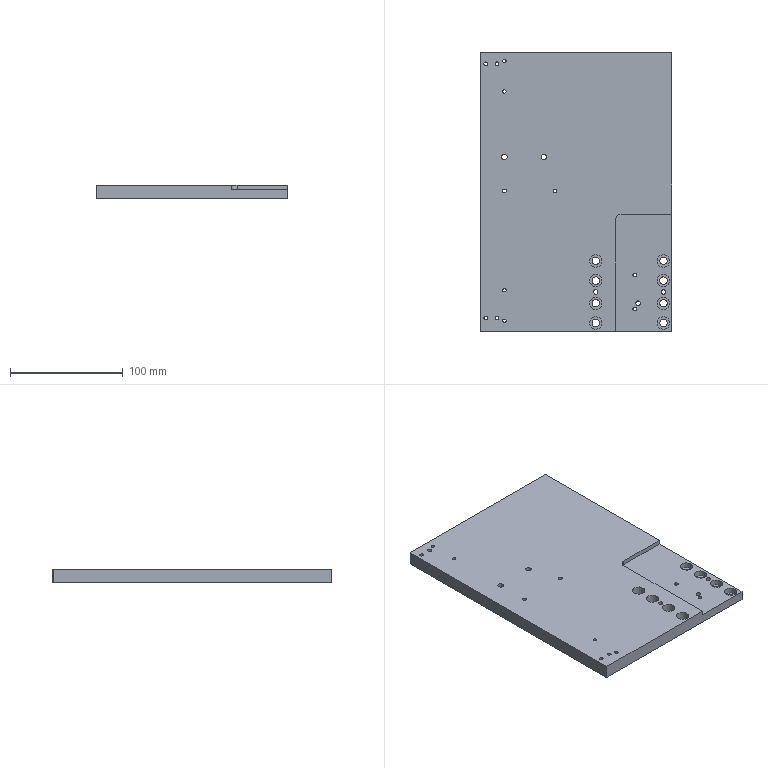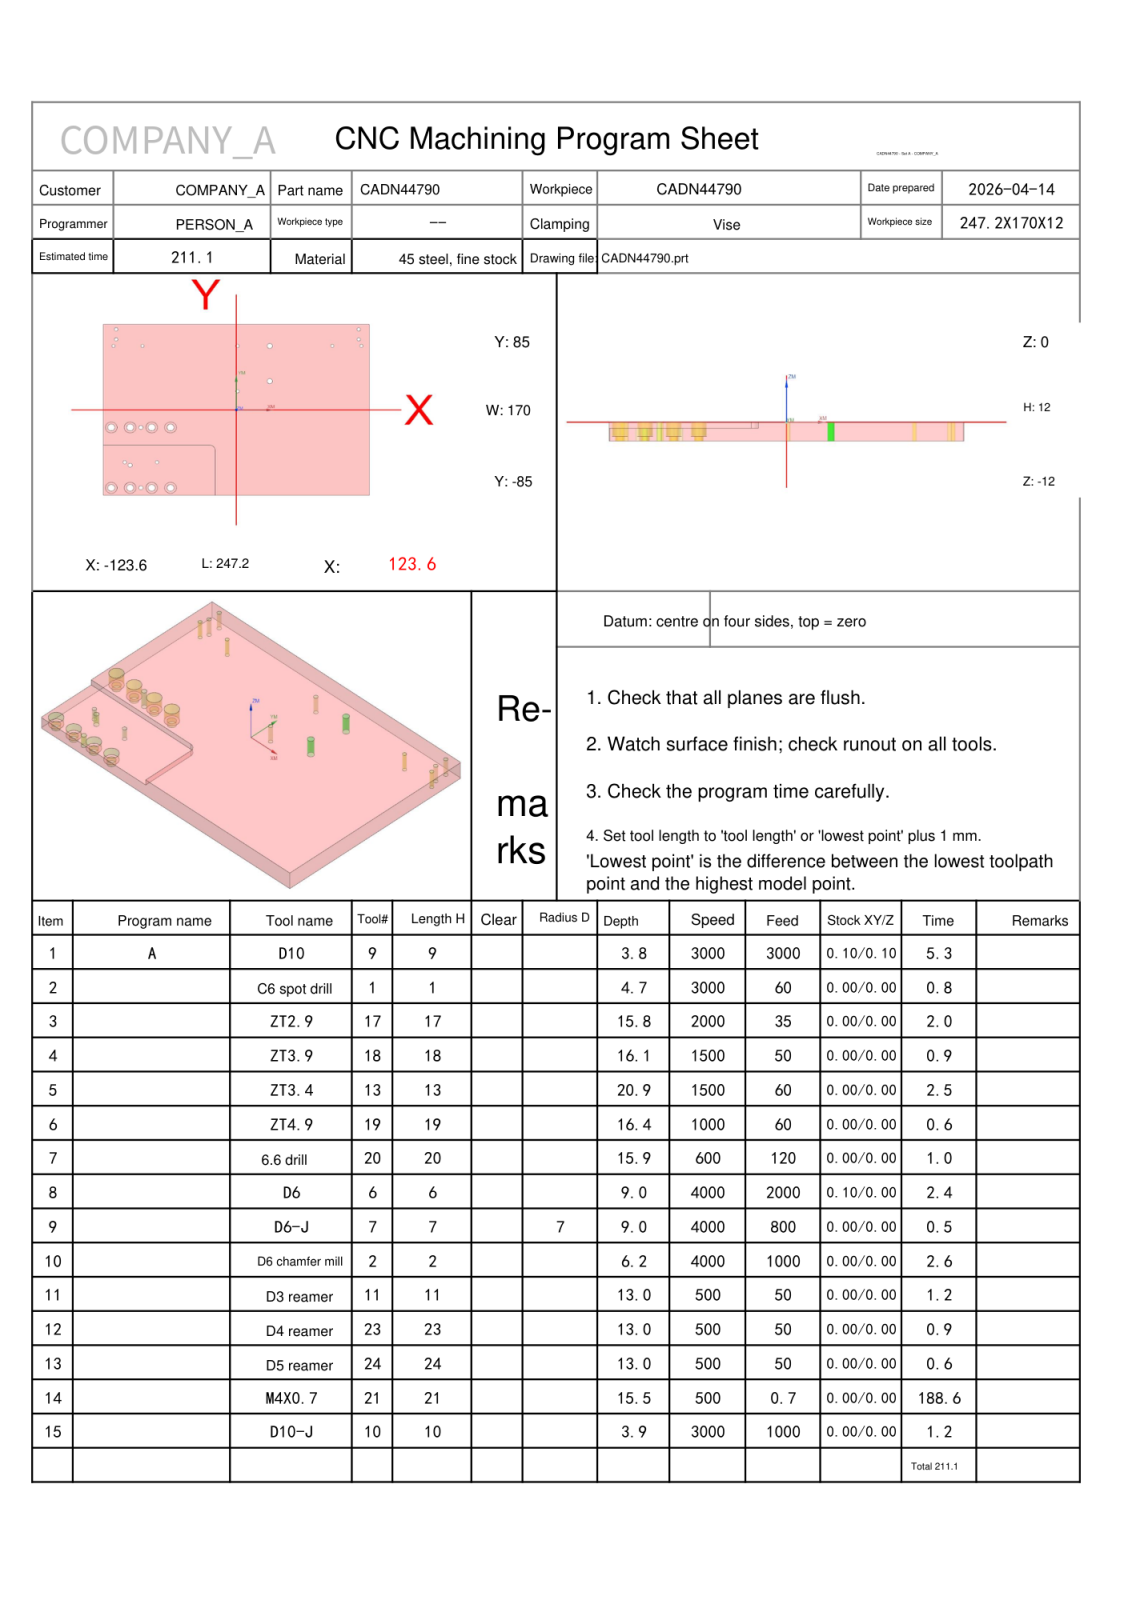NC program | NX | posted by the shop | part box 170 x 247.2 x 12 mm
Whole program, first 1507 of 2214 lines:
%
O0001
(Machine time: 390.98 MIN)
(===Total Tool:15===)
(T9=D10     D=10.  R=0.   D-  H09 Z=-3.8  )
(T1=C6 spot drill   D=6.   R=0.   D-  H01 Z=-4.7  )
(T17=ZT2.9  D=2.9  DR_a=120 D-  H17 Z=-15.84)
(T18=ZT3.9  D=3.9  DR_a=120 D-  H18 Z=-16.13)
(T13=ZT3.4  D=3.4  DR_a=118 D-  H13 Z=-20.9 )
(T19=ZT4.9  D=4.9  DR_a=120 D-  H19 Z=-16.41)
(T20=6.6 drill  D=6.6  DR_a=120 D-  H20 Z=-15.91)
(T6=D6      D=6.   R=0.   D-  H06 Z=-9.   )
(T7=D6-J    D=6.   R=0.   D7  H07 Z=-9.   )
(T2=D6 chamfer mill   D=6.   R=0.   D-  H02 Z=-6.2  )
(T11=D3 reamer   D=3.   DR_a=180 D-  H11 Z=-13.  )
(T23=D4 reamer   D=4.   DR_a=180 D-  H23 Z=-13.  )
(T24=D5 reamer   D=5.   DR_a=180 D-  H24 Z=-13.  )
(T21=M4X0.7 D=3.3  DR_a=180 D-  H21 Z=-15.5 )
(T10=D10-J  D=10.  R=0.   D10 H10 Z=-3.9  )
G80 G90 G17 G49 G40
G91 G28 Z0
M01
N1 T09 M06
(D10  D=10. R=0. H=09 ce=0.10 di=0.10)
G00 G90 G54 X-69.7 Y-93. M03 S3000
G43 H09 Z10.1
M08
Z1.3
G01 Z-.2 F3000.
Y-89.9
Y-86.195
G03 X-70.695 Y-85.2 I-1. J-.005
G01 X-127.501
G02 X-128.5 Y-84.201 I.001 J1.
G01 Y-78.699
G02 X-127.501 Y-77.7 I1. J-.001
G01 X-63.196
G02 X-62.2 Y-78.696 I-.004 J-1.
G01 Y-88.9
G03 X-61.2 Y-89.9 I1. J0.0
G01 X-55.7
G03 X-54.7 Y-88.9 I0.0 J1.
G01 Y-78.696
Y-71.196
G03 X-55.696 Y-70.2 I-1. J-.004
G01 X-127.501
G02 X-128.5 Y-69.201 I.001 J1.
G01 Y-63.699
G02 X-127.501 Y-62.7 I1. J-.001
G01 X-48.197
G02 X-47.2 Y-63.697 I-.003 J-1.
G01 Y-88.9
G03 X-46.2 Y-89.9 I1. J0.0
G01 X-40.7
G03 X-39.7 Y-88.9 I0.0 J1.
G01 Y-63.697
Y-56.197
G03 X-40.697 Y-55.2 I-1. J-.003
G01 X-127.501
G02 X-128.5 Y-54.201 I.001 J1.
G01 Y-48.699
G02 X-127.501 Y-47.7 I1. J-.001
G01 X-33.198
G02 X-32.2 Y-48.698 I-.002 J-1.
G01 Y-89.044
G03 X-31.354 Y-90.032 I1. J.001
G01 X-25.854 Y-90.888
X-25.7 Y-90.9
G03 X-24.7 Y-89.9 I0.0 J1.
G01 Y-40.2
X-128.5
X-131.7
Z1.3
G00 X-69.7 Y-93.
Z1.1
G01 Z-.4
Y-89.9
Y-86.195
G03 X-70.695 Y-85.2 I-1. J-.005
G01 X-127.501
G02 X-128.5 Y-84.201 I.001 J1.
G01 Y-78.699
G02 X-127.501 Y-77.7 I1. J-.001
G01 X-63.196
G02 X-62.2 Y-78.696 I-.004 J-1.
G01 Y-88.9
G03 X-61.2 Y-89.9 I1. J0.0
G01 X-55.7
G03 X-54.7 Y-88.9 I0.0 J1.
G01 Y-78.696
Y-71.196
G03 X-55.696 Y-70.2 I-1. J-.004
G01 X-127.501
G02 X-128.5 Y-69.201 I.001 J1.
G01 Y-63.699
G02 X-127.501 Y-62.7 I1. J-.001
G01 X-48.197
G02 X-47.2 Y-63.697 I-.003 J-1.
G01 Y-88.9
G03 X-46.2 Y-89.9 I1. J0.0
G01 X-40.7
G03 X-39.7 Y-88.9 I0.0 J1.
G01 Y-63.697
Y-56.197
G03 X-40.697 Y-55.2 I-1. J-.003
G01 X-127.501
G02 X-128.5 Y-54.201 I.001 J1.
G01 Y-48.699
G02 X-127.501 Y-47.7 I1. J-.001
G01 X-33.198
G02 X-32.2 Y-48.698 I-.002 J-1.
G01 Y-89.044
G03 X-31.354 Y-90.032 I1. J.001
G01 X-25.854 Y-90.888
X-25.7 Y-90.9
G03 X-24.7 Y-89.9 I0.0 J1.
G01 Y-40.2
X-128.5
X-131.7
Z1.1
G00 X-69.7 Y-93.
Z.9
G01 Z-.6
Y-89.9
Y-86.195
G03 X-70.695 Y-85.2 I-1. J-.005
G01 X-127.501
G02 X-128.5 Y-84.201 I.001 J1.
G01 Y-78.699
G02 X-127.501 Y-77.7 I1. J-.001
G01 X-63.196
G02 X-62.2 Y-78.696 I-.004 J-1.
G01 Y-88.9
G03 X-61.2 Y-89.9 I1. J0.0
G01 X-55.7
G03 X-54.7 Y-88.9 I0.0 J1.
G01 Y-78.696
Y-71.196
G03 X-55.696 Y-70.2 I-1. J-.004
G01 X-127.501
G02 X-128.5 Y-69.201 I.001 J1.
G01 Y-63.699
G02 X-127.501 Y-62.7 I1. J-.001
G01 X-48.197
G02 X-47.2 Y-63.697 I-.003 J-1.
G01 Y-88.9
G03 X-46.2 Y-89.9 I1. J0.0
G01 X-40.7
G03 X-39.7 Y-88.9 I0.0 J1.
G01 Y-63.697
Y-56.197
G03 X-40.697 Y-55.2 I-1. J-.003
G01 X-127.501
G02 X-128.5 Y-54.201 I.001 J1.
G01 Y-48.699
G02 X-127.501 Y-47.7 I1. J-.001
G01 X-33.198
G02 X-32.2 Y-48.698 I-.002 J-1.
G01 Y-89.044
G03 X-31.354 Y-90.032 I1. J.001
G01 X-25.854 Y-90.888
X-25.7 Y-90.9
G03 X-24.7 Y-89.9 I0.0 J1.
G01 Y-40.2
X-128.5
X-131.7
Z.9
G00 X-69.7 Y-93.
Z.7
G01 Z-.8
Y-89.9
Y-86.195
G03 X-70.695 Y-85.2 I-1. J-.005
G01 X-127.501
G02 X-128.5 Y-84.201 I.001 J1.
G01 Y-78.699
G02 X-127.501 Y-77.7 I1. J-.001
G01 X-63.196
G02 X-62.2 Y-78.696 I-.004 J-1.
G01 Y-88.9
G03 X-61.2 Y-89.9 I1. J0.0
G01 X-55.7
G03 X-54.7 Y-88.9 I0.0 J1.
G01 Y-78.696
Y-71.196
G03 X-55.696 Y-70.2 I-1. J-.004
G01 X-127.501
G02 X-128.5 Y-69.201 I.001 J1.
G01 Y-63.699
G02 X-127.501 Y-62.7 I1. J-.001
G01 X-48.197
G02 X-47.2 Y-63.697 I-.003 J-1.
G01 Y-88.9
G03 X-46.2 Y-89.9 I1. J0.0
G01 X-40.7
G03 X-39.7 Y-88.9 I0.0 J1.
G01 Y-63.697
Y-56.197
G03 X-40.697 Y-55.2 I-1. J-.003
G01 X-127.501
G02 X-128.5 Y-54.201 I.001 J1.
G01 Y-48.699
G02 X-127.501 Y-47.7 I1. J-.001
G01 X-33.198
G02 X-32.2 Y-48.698 I-.002 J-1.
G01 Y-89.044
G03 X-31.354 Y-90.032 I1. J.001
G01 X-25.854 Y-90.888
X-25.7 Y-90.9
G03 X-24.7 Y-89.9 I0.0 J1.
G01 Y-40.2
X-128.5
X-131.7
Z.7
G00 X-69.7 Y-93.
Z.5
G01 Z-1.
Y-89.9
Y-86.195
G03 X-70.695 Y-85.2 I-1. J-.005
G01 X-127.501
G02 X-128.5 Y-84.201 I.001 J1.
G01 Y-78.699
G02 X-127.501 Y-77.7 I1. J-.001
G01 X-63.196
G02 X-62.2 Y-78.696 I-.004 J-1.
G01 Y-88.9
G03 X-61.2 Y-89.9 I1. J0.0
G01 X-55.7
G03 X-54.7 Y-88.9 I0.0 J1.
G01 Y-78.696
Y-71.196
G03 X-55.696 Y-70.2 I-1. J-.004
G01 X-127.501
G02 X-128.5 Y-69.201 I.001 J1.
G01 Y-63.699
G02 X-127.501 Y-62.7 I1. J-.001
G01 X-48.197
G02 X-47.2 Y-63.697 I-.003 J-1.
G01 Y-88.9
G03 X-46.2 Y-89.9 I1. J0.0
G01 X-40.7
G03 X-39.7 Y-88.9 I0.0 J1.
G01 Y-63.697
Y-56.197
G03 X-40.697 Y-55.2 I-1. J-.003
G01 X-127.501
G02 X-128.5 Y-54.201 I.001 J1.
G01 Y-48.699
G02 X-127.501 Y-47.7 I1. J-.001
G01 X-33.198
G02 X-32.2 Y-48.698 I-.002 J-1.
G01 Y-89.044
G03 X-31.354 Y-90.032 I1. J.001
G01 X-25.854 Y-90.888
X-25.7 Y-90.9
G03 X-24.7 Y-89.9 I0.0 J1.
G01 Y-40.2
X-128.5
X-131.7
Z.5
G00 X-69.7 Y-93.
Z.3
G01 Z-1.2
Y-89.9
Y-86.195
G03 X-70.695 Y-85.2 I-1. J-.005
G01 X-127.501
G02 X-128.5 Y-84.201 I.001 J1.
G01 Y-78.699
G02 X-127.501 Y-77.7 I1. J-.001
G01 X-63.196
G02 X-62.2 Y-78.696 I-.004 J-1.
G01 Y-88.9
G03 X-61.2 Y-89.9 I1. J0.0
G01 X-55.7
G03 X-54.7 Y-88.9 I0.0 J1.
G01 Y-78.696
Y-71.196
G03 X-55.696 Y-70.2 I-1. J-.004
G01 X-127.501
G02 X-128.5 Y-69.201 I.001 J1.
G01 Y-63.699
G02 X-127.501 Y-62.7 I1. J-.001
G01 X-48.197
G02 X-47.2 Y-63.697 I-.003 J-1.
G01 Y-88.9
G03 X-46.2 Y-89.9 I1. J0.0
G01 X-40.7
G03 X-39.7 Y-88.9 I0.0 J1.
G01 Y-63.697
Y-56.197
G03 X-40.697 Y-55.2 I-1. J-.003
G01 X-127.501
G02 X-128.5 Y-54.201 I.001 J1.
G01 Y-48.699
G02 X-127.501 Y-47.7 I1. J-.001
G01 X-33.198
G02 X-32.2 Y-48.698 I-.002 J-1.
G01 Y-89.044
G03 X-31.354 Y-90.032 I1. J.001
G01 X-25.854 Y-90.888
X-25.7 Y-90.9
G03 X-24.7 Y-89.9 I0.0 J1.
G01 Y-40.2
X-128.5
X-131.7
Z.3
G00 X-69.7 Y-93.
Z.1
G01 Z-1.4
Y-89.9
Y-86.195
G03 X-70.695 Y-85.2 I-1. J-.005
G01 X-127.501
G02 X-128.5 Y-84.201 I.001 J1.
G01 Y-78.699
G02 X-127.501 Y-77.7 I1. J-.001
G01 X-63.196
G02 X-62.2 Y-78.696 I-.004 J-1.
G01 Y-88.9
G03 X-61.2 Y-89.9 I1. J0.0
G01 X-55.7
G03 X-54.7 Y-88.9 I0.0 J1.
G01 Y-78.696
Y-71.196
G03 X-55.696 Y-70.2 I-1. J-.004
G01 X-127.501
G02 X-128.5 Y-69.201 I.001 J1.
G01 Y-63.699
G02 X-127.501 Y-62.7 I1. J-.001
G01 X-48.197
G02 X-47.2 Y-63.697 I-.003 J-1.
G01 Y-88.9
G03 X-46.2 Y-89.9 I1. J0.0
G01 X-40.7
G03 X-39.7 Y-88.9 I0.0 J1.
G01 Y-63.697
Y-56.197
G03 X-40.697 Y-55.2 I-1. J-.003
G01 X-127.501
G02 X-128.5 Y-54.201 I.001 J1.
G01 Y-48.699
G02 X-127.501 Y-47.7 I1. J-.001
G01 X-33.198
G02 X-32.2 Y-48.698 I-.002 J-1.
G01 Y-89.044
G03 X-31.354 Y-90.032 I1. J.001
G01 X-25.854 Y-90.888
X-25.7 Y-90.9
G03 X-24.7 Y-89.9 I0.0 J1.
G01 Y-40.2
X-128.5
X-131.7
Z.1
G00 X-69.7 Y-93.
Z-.1
G01 Z-1.6
Y-89.9
Y-86.195
G03 X-70.695 Y-85.2 I-1. J-.005
G01 X-127.501
G02 X-128.5 Y-84.201 I.001 J1.
G01 Y-78.699
G02 X-127.501 Y-77.7 I1. J-.001
G01 X-63.196
G02 X-62.2 Y-78.696 I-.004 J-1.
G01 Y-88.9
G03 X-61.2 Y-89.9 I1. J0.0
G01 X-55.7
G03 X-54.7 Y-88.9 I0.0 J1.
G01 Y-78.696
Y-71.196
G03 X-55.696 Y-70.2 I-1. J-.004
G01 X-127.501
G02 X-128.5 Y-69.201 I.001 J1.
G01 Y-63.699
G02 X-127.501 Y-62.7 I1. J-.001
G01 X-48.197
G02 X-47.2 Y-63.697 I-.003 J-1.
G01 Y-88.9
G03 X-46.2 Y-89.9 I1. J0.0
G01 X-40.7
G03 X-39.7 Y-88.9 I0.0 J1.
G01 Y-63.697
Y-56.197
G03 X-40.697 Y-55.2 I-1. J-.003
G01 X-127.501
G02 X-128.5 Y-54.201 I.001 J1.
G01 Y-48.699
G02 X-127.501 Y-47.7 I1. J-.001
G01 X-33.198
G02 X-32.2 Y-48.698 I-.002 J-1.
G01 Y-89.044
G03 X-31.354 Y-90.032 I1. J.001
G01 X-25.854 Y-90.888
X-25.7 Y-90.9
G03 X-24.7 Y-89.9 I0.0 J1.
G01 Y-40.2
X-128.5
X-131.7
Z-.1
G00 X-69.7 Y-93.
Z-.3
G01 Z-1.8
Y-89.9
Y-86.195
G03 X-70.695 Y-85.2 I-1. J-.005
G01 X-127.501
G02 X-128.5 Y-84.201 I.001 J1.
G01 Y-78.699
G02 X-127.501 Y-77.7 I1. J-.001
G01 X-63.196
G02 X-62.2 Y-78.696 I-.004 J-1.
G01 Y-88.9
G03 X-61.2 Y-89.9 I1. J0.0
G01 X-55.7
G03 X-54.7 Y-88.9 I0.0 J1.
G01 Y-78.696
Y-71.196
G03 X-55.696 Y-70.2 I-1. J-.004
G01 X-127.501
G02 X-128.5 Y-69.201 I.001 J1.
G01 Y-63.699
G02 X-127.501 Y-62.7 I1. J-.001
G01 X-48.197
G02 X-47.2 Y-63.697 I-.003 J-1.
G01 Y-88.9
G03 X-46.2 Y-89.9 I1. J0.0
G01 X-40.7
G03 X-39.7 Y-88.9 I0.0 J1.
G01 Y-63.697
Y-56.197
G03 X-40.697 Y-55.2 I-1. J-.003
G01 X-127.501
G02 X-128.5 Y-54.201 I.001 J1.
G01 Y-48.699
G02 X-127.501 Y-47.7 I1. J-.001
G01 X-33.198
G02 X-32.2 Y-48.698 I-.002 J-1.
G01 Y-89.044
G03 X-31.354 Y-90.032 I1. J.001
G01 X-25.854 Y-90.888
X-25.7 Y-90.9
G03 X-24.7 Y-89.9 I0.0 J1.
G01 Y-40.2
X-128.5
X-131.7
Z-.3
G00 X-69.7 Y-93.
Z-.5
G01 Z-2.
Y-89.9
Y-86.195
G03 X-70.695 Y-85.2 I-1. J-.005
G01 X-127.501
G02 X-128.5 Y-84.201 I.001 J1.
G01 Y-78.699
G02 X-127.501 Y-77.7 I1. J-.001
G01 X-63.196
G02 X-62.2 Y-78.696 I-.004 J-1.
G01 Y-88.9
G03 X-61.2 Y-89.9 I1. J0.0
G01 X-55.7
G03 X-54.7 Y-88.9 I0.0 J1.
G01 Y-78.696
Y-71.196
G03 X-55.696 Y-70.2 I-1. J-.004
G01 X-127.501
G02 X-128.5 Y-69.201 I.001 J1.
G01 Y-63.699
G02 X-127.501 Y-62.7 I1. J-.001
G01 X-48.197
G02 X-47.2 Y-63.697 I-.003 J-1.
G01 Y-88.9
G03 X-46.2 Y-89.9 I1. J0.0
G01 X-40.7
G03 X-39.7 Y-88.9 I0.0 J1.
G01 Y-63.697
Y-56.197
G03 X-40.697 Y-55.2 I-1. J-.003
G01 X-127.501
G02 X-128.5 Y-54.201 I.001 J1.
G01 Y-48.699
G02 X-127.501 Y-47.7 I1. J-.001
G01 X-33.198
G02 X-32.2 Y-48.698 I-.002 J-1.
G01 Y-89.044
G03 X-31.354 Y-90.032 I1. J.001
G01 X-25.854 Y-90.888
X-25.7 Y-90.9
G03 X-24.7 Y-89.9 I0.0 J1.
G01 Y-40.2
X-128.5
X-131.7
Z-.5
G00 X-69.7 Y-93.
Z-.7
G01 Z-2.2
Y-89.9
Y-86.195
G03 X-70.695 Y-85.2 I-1. J-.005
G01 X-127.501
G02 X-128.5 Y-84.201 I.001 J1.
G01 Y-78.699
G02 X-127.501 Y-77.7 I1. J-.001
G01 X-63.196
G02 X-62.2 Y-78.696 I-.004 J-1.
G01 Y-88.9
G03 X-61.2 Y-89.9 I1. J0.0
G01 X-55.7
G03 X-54.7 Y-88.9 I0.0 J1.
G01 Y-78.696
Y-71.196
G03 X-55.696 Y-70.2 I-1. J-.004
G01 X-127.501
G02 X-128.5 Y-69.201 I.001 J1.
G01 Y-63.699
G02 X-127.501 Y-62.7 I1. J-.001
G01 X-48.197
G02 X-47.2 Y-63.697 I-.003 J-1.
G01 Y-88.9
G03 X-46.2 Y-89.9 I1. J0.0
G01 X-40.7
G03 X-39.7 Y-88.9 I0.0 J1.
G01 Y-63.697
Y-56.197
G03 X-40.697 Y-55.2 I-1. J-.003
G01 X-127.501
G02 X-128.5 Y-54.201 I.001 J1.
G01 Y-48.699
G02 X-127.501 Y-47.7 I1. J-.001
G01 X-33.198
G02 X-32.2 Y-48.698 I-.002 J-1.
G01 Y-89.044
G03 X-31.354 Y-90.032 I1. J.001
G01 X-25.854 Y-90.888
X-25.7 Y-90.9
G03 X-24.7 Y-89.9 I0.0 J1.
G01 Y-40.2
X-128.5
X-131.7
Z-.7
G00 X-69.7 Y-93.
Z-.9
G01 Z-2.4
Y-89.9
Y-86.195
G03 X-70.695 Y-85.2 I-1. J-.005
G01 X-127.501
G02 X-128.5 Y-84.201 I.001 J1.
G01 Y-78.699
G02 X-127.501 Y-77.7 I1. J-.001
G01 X-63.196
G02 X-62.2 Y-78.696 I-.004 J-1.
G01 Y-88.9
G03 X-61.2 Y-89.9 I1. J0.0
G01 X-55.7
G03 X-54.7 Y-88.9 I0.0 J1.
G01 Y-78.696
Y-71.196
G03 X-55.696 Y-70.2 I-1. J-.004
G01 X-127.501
G02 X-128.5 Y-69.201 I.001 J1.
G01 Y-63.699
G02 X-127.501 Y-62.7 I1. J-.001
G01 X-48.197
G02 X-47.2 Y-63.697 I-.003 J-1.
G01 Y-88.9
G03 X-46.2 Y-89.9 I1. J0.0
G01 X-40.7
G03 X-39.7 Y-88.9 I0.0 J1.
G01 Y-63.697
Y-56.197
G03 X-40.697 Y-55.2 I-1. J-.003
G01 X-127.501
G02 X-128.5 Y-54.201 I.001 J1.
G01 Y-48.699
G02 X-127.501 Y-47.7 I1. J-.001
G01 X-33.198
G02 X-32.2 Y-48.698 I-.002 J-1.
G01 Y-89.044
G03 X-31.354 Y-90.032 I1. J.001
G01 X-25.854 Y-90.888
X-25.7 Y-90.9
G03 X-24.7 Y-89.9 I0.0 J1.
G01 Y-40.2
X-128.5
X-131.7
Z-.9
G00 X-69.7 Y-93.
Z-1.1
G01 Z-2.6
Y-89.9
Y-86.195
G03 X-70.695 Y-85.2 I-1. J-.005
G01 X-127.501
G02 X-128.5 Y-84.201 I.001 J1.
G01 Y-78.699
G02 X-127.501 Y-77.7 I1. J-.001
G01 X-63.196
G02 X-62.2 Y-78.696 I-.004 J-1.
G01 Y-88.9
G03 X-61.2 Y-89.9 I1. J0.0
G01 X-55.7
G03 X-54.7 Y-88.9 I0.0 J1.
G01 Y-78.696
Y-71.196
G03 X-55.696 Y-70.2 I-1. J-.004
G01 X-127.501
G02 X-128.5 Y-69.201 I.001 J1.
G01 Y-63.699
G02 X-127.501 Y-62.7 I1. J-.001
G01 X-48.197
G02 X-47.2 Y-63.697 I-.003 J-1.
G01 Y-88.9
G03 X-46.2 Y-89.9 I1. J0.0
G01 X-40.7
G03 X-39.7 Y-88.9 I0.0 J1.
G01 Y-63.697
Y-56.197
G03 X-40.697 Y-55.2 I-1. J-.003
G01 X-127.501
G02 X-128.5 Y-54.201 I.001 J1.
G01 Y-48.699
G02 X-127.501 Y-47.7 I1. J-.001
G01 X-33.198
G02 X-32.2 Y-48.698 I-.002 J-1.
G01 Y-89.044
G03 X-31.354 Y-90.032 I1. J.001
G01 X-25.854 Y-90.888
X-25.7 Y-90.9
G03 X-24.7 Y-89.9 I0.0 J1.
G01 Y-40.2
X-128.5
X-131.7
Z-1.1
G00 X-69.7 Y-93.
Z-1.3
G01 Z-2.8
Y-89.9
Y-86.195
G03 X-70.695 Y-85.2 I-1. J-.005
G01 X-127.501
G02 X-128.5 Y-84.201 I.001 J1.
G01 Y-78.699
G02 X-127.501 Y-77.7 I1. J-.001
G01 X-63.196
G02 X-62.2 Y-78.696 I-.004 J-1.
G01 Y-88.9
G03 X-61.2 Y-89.9 I1. J0.0
G01 X-55.7
G03 X-54.7 Y-88.9 I0.0 J1.
G01 Y-78.696
Y-71.196
G03 X-55.696 Y-70.2 I-1. J-.004
G01 X-127.501
G02 X-128.5 Y-69.201 I.001 J1.
G01 Y-63.699
G02 X-127.501 Y-62.7 I1. J-.001
G01 X-48.197
G02 X-47.2 Y-63.697 I-.003 J-1.
G01 Y-88.9
G03 X-46.2 Y-89.9 I1. J0.0
G01 X-40.7
G03 X-39.7 Y-88.9 I0.0 J1.
G01 Y-63.697
Y-56.197
G03 X-40.697 Y-55.2 I-1. J-.003
G01 X-127.501
G02 X-128.5 Y-54.201 I.001 J1.
G01 Y-48.699
G02 X-127.501 Y-47.7 I1. J-.001
G01 X-33.198
G02 X-32.2 Y-48.698 I-.002 J-1.
G01 Y-89.044
G03 X-31.354 Y-90.032 I1. J.001
G01 X-25.854 Y-90.888
X-25.7 Y-90.9
G03 X-24.7 Y-89.9 I0.0 J1.
G01 Y-40.2
X-128.5
X-131.7
Z-1.3
G00 X-69.7 Y-93.
Z-1.5
G01 Z-3.
Y-89.9
Y-86.195
G03 X-70.695 Y-85.2 I-1. J-.005
G01 X-127.501
G02 X-128.5 Y-84.201 I.001 J1.
G01 Y-78.699
G02 X-127.501 Y-77.7 I1. J-.001
G01 X-63.196
G02 X-62.2 Y-78.696 I-.004 J-1.
G01 Y-88.9
G03 X-61.2 Y-89.9 I1. J0.0
G01 X-55.7
G03 X-54.7 Y-88.9 I0.0 J1.
G01 Y-78.696
Y-71.196
G03 X-55.696 Y-70.2 I-1. J-.004
G01 X-127.501
G02 X-128.5 Y-69.201 I.001 J1.
G01 Y-63.699
G02 X-127.501 Y-62.7 I1. J-.001
G01 X-48.197
G02 X-47.2 Y-63.697 I-.003 J-1.
G01 Y-88.9
G03 X-46.2 Y-89.9 I1. J0.0
G01 X-40.7
G03 X-39.7 Y-88.9 I0.0 J1.
G01 Y-63.697
Y-56.197
G03 X-40.697 Y-55.2 I-1. J-.003
G01 X-127.501
G02 X-128.5 Y-54.201 I.001 J1.
G01 Y-48.699
G02 X-127.501 Y-47.7 I1. J-.001
G01 X-33.198
G02 X-32.2 Y-48.698 I-.002 J-1.
G01 Y-89.044
G03 X-31.354 Y-90.032 I1. J.001
G01 X-25.854 Y-90.888
X-25.7 Y-90.9
G03 X-24.7 Y-89.9 I0.0 J1.
G01 Y-40.2
X-128.5
X-131.7
Z-1.5
G00 X-69.7 Y-93.
Z-1.7
G01 Z-3.2
Y-89.9
Y-86.195
G03 X-70.695 Y-85.2 I-1. J-.005
G01 X-127.501
G02 X-128.5 Y-84.201 I.001 J1.
G01 Y-78.699
G02 X-127.501 Y-77.7 I1. J-.001
G01 X-63.196
G02 X-62.2 Y-78.696 I-.004 J-1.
G01 Y-88.9
G03 X-61.2 Y-89.9 I1. J0.0
G01 X-55.7
G03 X-54.7 Y-88.9 I0.0 J1.
G01 Y-78.696
Y-71.196
G03 X-55.696 Y-70.2 I-1. J-.004
G01 X-127.501
G02 X-128.5 Y-69.201 I.001 J1.
G01 Y-63.699
G02 X-127.501 Y-62.7 I1. J-.001
G01 X-48.197
G02 X-47.2 Y-63.697 I-.003 J-1.
G01 Y-88.9
G03 X-46.2 Y-89.9 I1. J0.0
G01 X-40.7
G03 X-39.7 Y-88.9 I0.0 J1.
G01 Y-63.697
Y-56.197
G03 X-40.697 Y-55.2 I-1. J-.003
G01 X-127.501
G02 X-128.5 Y-54.201 I.001 J1.
G01 Y-48.699
G02 X-127.501 Y-47.7 I1. J-.001
G01 X-33.198
G02 X-32.2 Y-48.698 I-.002 J-1.
G01 Y-89.044
G03 X-31.354 Y-90.032 I1. J.001
G01 X-25.854 Y-90.888
X-25.7 Y-90.9
G03 X-24.7 Y-89.9 I0.0 J1.
G01 Y-40.2
X-128.5
X-131.7
Z-1.7
G00 X-69.7 Y-93.
Z-1.9
G01 Z-3.4
Y-89.9
Y-86.195
G03 X-70.695 Y-85.2 I-1. J-.005
G01 X-127.501
G02 X-128.5 Y-84.201 I.001 J1.
G01 Y-78.699
G02 X-127.501 Y-77.7 I1. J-.001
G01 X-63.196
G02 X-62.2 Y-78.696 I-.004 J-1.
G01 Y-88.9
G03 X-61.2 Y-89.9 I1. J0.0
G01 X-55.7
G03 X-54.7 Y-88.9 I0.0 J1.
G01 Y-78.696
Y-71.196
G03 X-55.696 Y-70.2 I-1. J-.004
G01 X-127.501
G02 X-128.5 Y-69.201 I.001 J1.
G01 Y-63.699
G02 X-127.501 Y-62.7 I1. J-.001
G01 X-48.197
G02 X-47.2 Y-63.697 I-.003 J-1.
G01 Y-88.9
G03 X-46.2 Y-89.9 I1. J0.0
G01 X-40.7
G03 X-39.7 Y-88.9 I0.0 J1.
G01 Y-63.697
Y-56.197
G03 X-40.697 Y-55.2 I-1. J-.003
G01 X-127.501
G02 X-128.5 Y-54.201 I.001 J1.
G01 Y-48.699
G02 X-127.501 Y-47.7 I1. J-.001
G01 X-33.198
G02 X-32.2 Y-48.698 I-.002 J-1.
G01 Y-89.044
G03 X-31.354 Y-90.032 I1. J.001
G01 X-25.854 Y-90.888
X-25.7 Y-90.9
G03 X-24.7 Y-89.9 I0.0 J1.
G01 Y-40.2
X-128.5
X-131.7
Z-1.9
G00 X-69.7 Y-93.
Z-2.1
G01 Z-3.6
Y-89.9
Y-86.195
G03 X-70.695 Y-85.2 I-1. J-.005
G01 X-127.501
G02 X-128.5 Y-84.201 I.001 J1.
G01 Y-78.699
G02 X-127.501 Y-77.7 I1. J-.001
G01 X-63.196
G02 X-62.2 Y-78.696 I-.004 J-1.
G01 Y-88.9
G03 X-61.2 Y-89.9 I1. J0.0
G01 X-55.7
G03 X-54.7 Y-88.9 I0.0 J1.
G01 Y-78.696
Y-71.196
G03 X-55.696 Y-70.2 I-1. J-.004
G01 X-127.501
G02 X-128.5 Y-69.201 I.001 J1.
G01 Y-63.699
G02 X-127.501 Y-62.7 I1. J-.001
G01 X-48.197
G02 X-47.2 Y-63.697 I-.003 J-1.
G01 Y-88.9
G03 X-46.2 Y-89.9 I1. J0.0
G01 X-40.7
G03 X-39.7 Y-88.9 I0.0 J1.
G01 Y-63.697
Y-56.197
G03 X-40.697 Y-55.2 I-1. J-.003
G01 X-127.501
G02 X-128.5 Y-54.201 I.001 J1.
G01 Y-48.699
G02 X-127.501 Y-47.7 I1. J-.001
G01 X-33.198
G02 X-32.2 Y-48.698 I-.002 J-1.
G01 Y-89.044
G03 X-31.354 Y-90.032 I1. J.001
G01 X-25.854 Y-90.888
X-25.7 Y-90.9
G03 X-24.7 Y-89.9 I0.0 J1.
G01 Y-40.2
X-128.5
X-131.7
Z-2.1
G00 X-69.7 Y-93.
Z-2.3
G01 Z-3.8
Y-89.9
Y-86.195
G03 X-70.695 Y-85.2 I-1. J-.005
G01 X-127.501
G02 X-128.5 Y-84.201 I.001 J1.
G01 Y-78.699
G02 X-127.501 Y-77.7 I1. J-.001
G01 X-63.196
G02 X-62.2 Y-78.696 I-.004 J-1.
G01 Y-88.9
G03 X-61.2 Y-89.9 I1. J0.0
G01 X-55.7
G03 X-54.7 Y-88.9 I0.0 J1.
G01 Y-78.696
Y-71.196
G03 X-55.696 Y-70.2 I-1. J-.004
G01 X-127.501
G02 X-128.5 Y-69.201 I.001 J1.
G01 Y-63.699
G02 X-127.501 Y-62.7 I1. J-.001
G01 X-48.197
G02 X-47.2 Y-63.697 I-.003 J-1.
G01 Y-88.9
G03 X-46.2 Y-89.9 I1. J0.0
G01 X-40.7
G03 X-39.7 Y-88.9 I0.0 J1.
G01 Y-63.697
Y-56.197
G03 X-40.697 Y-55.2 I-1. J-.003
G01 X-127.501
G02 X-128.5 Y-54.201 I.001 J1.
G01 Y-48.699
G02 X-127.501 Y-47.7 I1. J-.001
G01 X-33.198
G02 X-32.2 Y-48.698 I-.002 J-1.
G01 Y-89.044
G03 X-31.354 Y-90.032 I1. J.001
G01 X-25.854 Y-90.888
X-25.7 Y-90.9
G03 X-24.7 Y-89.9 I0.0 J1.
G01 Y-40.2
X-128.5
X-131.7
Z-2.3
G00 Z10.1
G91 G28 Z0.0
M05
M09
G91 G28 Z0.0
M01
N2 T01 M06
(C6 spot drill  D=6. R=0. H=01 ce=0.00 di=0.10)
G00 G90 G54 X-111.6 Y80. M03 S3000
G43 H01 Z20.
M08
G98 G81 X-111.6 Y80. Z-.8 R1. F60.
Y70.
X-114.1 Y63.5
X-87.1
X-78.6 Y-17.5
X-88.6
X-98.6
X-116.1
X-103.6 Y-52. Z-4.7 R-2.9
X-98.6 Y-55.
X-116.1 Y-77.5
X-98.6
X-88.6
X-78.6
X-61.1
X-73.6 Y-52.
X-61.1 Y-17.5 Z-.8 R1.
X1. Y18.5
X31. Y28.5
X1. Y63.5
X31.
X89.1
X116.1
X113.6 Y70.
Y80.
G80
G00 Z20.
G91 G28 Z0.0
M05
M09
G91 G28 Z0.0
M01
N3 T17 M06
(ZT2.9 D=2.9 DR_a=120 H=17)
G00 G90 G54 X116.1 Y63.5 M03 S2000
G43 H17 Z20.
M08
G98 G83 X116.1 Y63.5 Z-15.837 R1. F35. Q1.
X89.1
X-87.1
X-114.1
G80
G00 Z20.
G91 G28 Z0.0
M05
M09
G91 G28 Z0.0
M01
N4 T18 M06
(ZT3.9 D=3.9 DR_a=120 H=18)
G00 G90 G54 X-88.6 Y-17.5 M03 S1500
G43 H18 Z20.
M08
G98 G83 X-88.6 Y-17.5 Z-16.126 R1. F50. Q1.
G98 G83 X-98.6 Y-55. Z-16.126 R-2.9 Q1.
X-88.6 Y-77.5
G80
G00 Z20.
G91 G28 Z0.0
M05
M09
G91 G28 Z0.0
M01
N5 T13 M06
(ZT3.4 D=3.4 DR_a=118 H=13)
G00 G90 G54 X113.6 Y80. M03 S1500
G43 H13 Z20.
M08
G98 G83 X113.6 Y80. Z-17. R1. F60. Q1.
Y70.
X1. Y63.5
Y18.5
X-73.6 Y-52. Z-20.9 R-2.9
X-103.6
X-111.6 Y70. Z-17. R1.
Y80.
G80
G00 Z20.
G91 G28 Z0.0
M05
M09
G91 G28 Z0.0
M01
N6 T19 M06
(ZT4.9 D=4.9 DR_a=120 H=19)
G00 G90 G54 X31. Y63.5 M03 S1000
G43 H19 Z20.
M08
G98 G83 X31. Y63.5 Z-16.415 R1. F60. Q1.
Y28.5
G80
G00 Z20.
G91 G28 Z0.0
M05
M09
G91 G28 Z0.0
M01
N7 T20 M06
(6.6 drill D=6.6 DR_a=120 H=20)
G00 G90 G54 X-116.1 Y-77.5 M03 S600
G43 H20 Z20.
M08
G98 G83 X-116.1 Y-77.5 Z-15.905 R-2.9 F120. Q2.
X-98.6
X-78.6
X-61.1
G98 G83 X-61.1 Y-17.5 Z-15.905 R1. Q2.
X-78.6
X-98.6
X-116.1
G80
G00 Z20.
G91 G28 Z0.0
M05
M09
G91 G28 Z0.0
M01
N8 T06 M06
(D6  D=6. R=0. H=06 ce=0.10 di=0.00)
G00 G90 G54 X-78.6 Y-17.5 M03 S4000
G43 H06 Z20.
M08
Z.5
G03 X-79.8 Y-18.7 I0.0 J-1.2 F2000.
X-78.6 Y-19.9 I1.2 J0.0
X-78.6 Y-19.9 Z.3 I0.0 J2.4
X-78.6 Y-19.9 Z.1 I0.0 J2.4
X-78.6 Y-19.9 Z-.1 I0.0 J2.4
X-78.6 Y-19.9 Z-.3 I0.0 J2.4
X-78.6 Y-19.9 Z-.5 I0.0 J2.4
X-78.6 Y-19.9 Z-.7 I0.0 J2.4
X-78.6 Y-19.9 Z-.9 I0.0 J2.4
X-78.6 Y-19.9 Z-1.1 I0.0 J2.4
X-78.6 Y-19.9 Z-1.3 I0.0 J2.4
X-78.6 Y-19.9 Z-1.5 I0.0 J2.4
X-78.6 Y-19.9 Z-1.7 I0.0 J2.4
X-78.6 Y-19.9 Z-1.9 I0.0 J2.4
X-78.6 Y-19.9 Z-2.1 I0.0 J2.4
X-78.6 Y-19.9 Z-2.3 I0.0 J2.4
X-78.6 Y-19.9 Z-2.5 I0.0 J2.4
X-78.6 Y-19.9 Z-2.7 I0.0 J2.4
X-78.6 Y-19.9 Z-2.9 I0.0 J2.4
X-78.6 Y-19.9 Z-3.1 I0.0 J2.4
X-78.6 Y-19.9 Z-3.3 I0.0 J2.4
X-78.6 Y-19.9 Z-3.5 I0.0 J2.4
X-78.6 Y-19.9 Z-3.7 I0.0 J2.4
X-78.6 Y-19.9 Z-3.9 I0.0 J2.4
X-78.6 Y-19.9 Z-4.1 I0.0 J2.4
X-78.6 Y-19.9 Z-4.3 I0.0 J2.4
X-78.6 Y-19.9 Z-4.5 I0.0 J2.4
X-78.6 Y-19.9 Z-4.7 I0.0 J2.4
X-78.6 Y-19.9 Z-4.9 I0.0 J2.4
X-78.6 Y-19.9 Z-5.1 I0.0 J2.4
X-78.6 Y-19.9 Z-5.3 I0.0 J2.4
X-78.6 Y-19.9 Z-5.5 I0.0 J2.4
X-78.6 Y-19.9 Z-5.7 I0.0 J2.4
X-78.6 Y-19.9 Z-5.9 I0.0 J2.4
X-78.6 Y-19.9 Z-6.1 I0.0 J2.4
X-78.6 Y-19.9 Z-6.3 I0.0 J2.4
X-78.6 Y-19.9 Z-6.5 I0.0 J2.4
X-78.6 Y-19.9 Z-6.7 I0.0 J2.4
X-78.6 Y-19.9 Z-6.9 I0.0 J2.4
X-78.6 Y-19.9 Z-7.1 I0.0 J2.4
X-78.6 Y-19.9 Z-7.3 I0.0 J2.4
X-78.6 Y-19.9 Z-7.5 I0.0 J2.4
X-78.6 Y-19.9 Z-7.7 I0.0 J2.4
X-78.6 Y-19.9 Z-7.9 I0.0 J2.4
X-78.6 Y-19.9 Z-8.1 I0.0 J2.4
X-78.6 Y-19.9 Z-8.3 I0.0 J2.4
X-78.6 Y-19.9 Z-8.5 I0.0 J2.4
X-78.6 Y-19.9 Z-8.7 I0.0 J2.4
X-78.6 Y-19.9 Z-8.9 I0.0 J2.4
X-78.6 Y-15.1 Z-9. I0.0 J2.4
X-81. Y-17.5 I0.0 J-2.4
X-78.6 Y-19.9 I2.4 J0.0
X-76.2 Y-17.5 I0.0 J2.4
X-78.6 Y-15.1 I-2.4 J0.0
X-79.8 Y-16.3 I0.0 J-1.2
X-78.6 Y-17.5 I1.2 J0.0
G00 Z20.
X-61.1
Z.5
G03 X-62.3 Y-18.7 I0.0 J-1.2
X-61.1 Y-19.9 I1.2 J0.0
X-61.1 Y-19.9 Z.3 I0.0 J2.4
X-61.1 Y-19.9 Z.1 I0.0 J2.4
X-61.1 Y-19.9 Z-.1 I0.0 J2.4
X-61.1 Y-19.9 Z-.3 I0.0 J2.4
X-61.1 Y-19.9 Z-.5 I0.0 J2.4
X-61.1 Y-19.9 Z-.7 I0.0 J2.4
X-61.1 Y-19.9 Z-.9 I0.0 J2.4
X-61.1 Y-19.9 Z-1.1 I0.0 J2.4
X-61.1 Y-19.9 Z-1.3 I0.0 J2.4
X-61.1 Y-19.9 Z-1.5 I0.0 J2.4
X-61.1 Y-19.9 Z-1.7 I0.0 J2.4
X-61.1 Y-19.9 Z-1.9 I0.0 J2.4
X-61.1 Y-19.9 Z-2.1 I0.0 J2.4
X-61.1 Y-19.9 Z-2.3 I0.0 J2.4
X-61.1 Y-19.9 Z-2.5 I0.0 J2.4
X-61.1 Y-19.9 Z-2.7 I0.0 J2.4
X-61.1 Y-19.9 Z-2.9 I0.0 J2.4
X-61.1 Y-19.9 Z-3.1 I0.0 J2.4
X-61.1 Y-19.9 Z-3.3 I0.0 J2.4
X-61.1 Y-19.9 Z-3.5 I0.0 J2.4
X-61.1 Y-19.9 Z-3.7 I0.0 J2.4
X-61.1 Y-19.9 Z-3.9 I0.0 J2.4
X-61.1 Y-19.9 Z-4.1 I0.0 J2.4
X-61.1 Y-19.9 Z-4.3 I0.0 J2.4
X-61.1 Y-19.9 Z-4.5 I0.0 J2.4
X-61.1 Y-19.9 Z-4.7 I0.0 J2.4
X-61.1 Y-19.9 Z-4.9 I0.0 J2.4
X-61.1 Y-19.9 Z-5.1 I0.0 J2.4
X-61.1 Y-19.9 Z-5.3 I0.0 J2.4
X-61.1 Y-19.9 Z-5.5 I0.0 J2.4
X-61.1 Y-19.9 Z-5.7 I0.0 J2.4
X-61.1 Y-19.9 Z-5.9 I0.0 J2.4
X-61.1 Y-19.9 Z-6.1 I0.0 J2.4
X-61.1 Y-19.9 Z-6.3 I0.0 J2.4
X-61.1 Y-19.9 Z-6.5 I0.0 J2.4
X-61.1 Y-19.9 Z-6.7 I0.0 J2.4
X-61.1 Y-19.9 Z-6.9 I0.0 J2.4
X-61.1 Y-19.9 Z-7.1 I0.0 J2.4
X-61.1 Y-19.9 Z-7.3 I0.0 J2.4
X-61.1 Y-19.9 Z-7.5 I0.0 J2.4
X-61.1 Y-19.9 Z-7.7 I0.0 J2.4
X-61.1 Y-19.9 Z-7.9 I0.0 J2.4
X-61.1 Y-19.9 Z-8.1 I0.0 J2.4
X-61.1 Y-19.9 Z-8.3 I0.0 J2.4
X-61.1 Y-19.9 Z-8.5 I0.0 J2.4
X-61.1 Y-19.9 Z-8.7 I0.0 J2.4
X-61.1 Y-19.9 Z-8.9 I0.0 J2.4
X-61.1 Y-15.1 Z-9. I0.0 J2.4
X-63.5 Y-17.5 I0.0 J-2.4
X-61.1 Y-19.9 I2.4 J0.0
X-58.7 Y-17.5 I0.0 J2.4
X-61.1 Y-15.1 I-2.4 J0.0
X-62.3 Y-16.3 I0.0 J-1.2
X-61.1 Y-17.5 I1.2 J0.0
G00 Z20.
X-98.6
Z.5
G03 X-99.8 Y-18.7 I0.0 J-1.2
X-98.6 Y-19.9 I1.2 J0.0
X-98.6 Y-19.9 Z.3 I0.0 J2.4
X-98.6 Y-19.9 Z.1 I0.0 J2.4
X-98.6 Y-19.9 Z-.1 I0.0 J2.4
X-98.6 Y-19.9 Z-.3 I0.0 J2.4
X-98.6 Y-19.9 Z-.5 I0.0 J2.4
X-98.6 Y-19.9 Z-.7 I0.0 J2.4
X-98.6 Y-19.9 Z-.9 I0.0 J2.4
X-98.6 Y-19.9 Z-1.1 I0.0 J2.4
X-98.6 Y-19.9 Z-1.3 I0.0 J2.4
X-98.6 Y-19.9 Z-1.5 I0.0 J2.4
X-98.6 Y-19.9 Z-1.7 I0.0 J2.4
X-98.6 Y-19.9 Z-1.9 I0.0 J2.4
X-98.6 Y-19.9 Z-2.1 I0.0 J2.4
X-98.6 Y-19.9 Z-2.3 I0.0 J2.4
X-98.6 Y-19.9 Z-2.5 I0.0 J2.4
X-98.6 Y-19.9 Z-2.7 I0.0 J2.4
X-98.6 Y-19.9 Z-2.9 I0.0 J2.4
X-98.6 Y-19.9 Z-3.1 I0.0 J2.4
X-98.6 Y-19.9 Z-3.3 I0.0 J2.4
X-98.6 Y-19.9 Z-3.5 I0.0 J2.4
X-98.6 Y-19.9 Z-3.7 I0.0 J2.4
X-98.6 Y-19.9 Z-3.9 I0.0 J2.4
X-98.6 Y-19.9 Z-4.1 I0.0 J2.4
X-98.6 Y-19.9 Z-4.3 I0.0 J2.4
X-98.6 Y-19.9 Z-4.5 I0.0 J2.4
X-98.6 Y-19.9 Z-4.7 I0.0 J2.4
X-98.6 Y-19.9 Z-4.9 I0.0 J2.4
X-98.6 Y-19.9 Z-5.1 I0.0 J2.4
X-98.6 Y-19.9 Z-5.3 I0.0 J2.4
X-98.6 Y-19.9 Z-5.5 I0.0 J2.4
X-98.6 Y-19.9 Z-5.7 I0.0 J2.4
X-98.6 Y-19.9 Z-5.9 I0.0 J2.4
X-98.6 Y-19.9 Z-6.1 I0.0 J2.4
X-98.6 Y-19.9 Z-6.3 I0.0 J2.4
X-98.6 Y-19.9 Z-6.5 I0.0 J2.4
X-98.6 Y-19.9 Z-6.7 I0.0 J2.4
X-98.6 Y-19.9 Z-6.9 I0.0 J2.4
X-98.6 Y-19.9 Z-7.1 I0.0 J2.4
X-98.6 Y-19.9 Z-7.3 I0.0 J2.4
X-98.6 Y-19.9 Z-7.5 I0.0 J2.4
X-98.6 Y-19.9 Z-7.7 I0.0 J2.4
X-98.6 Y-19.9 Z-7.9 I0.0 J2.4
X-98.6 Y-19.9 Z-8.1 I0.0 J2.4
X-98.6 Y-19.9 Z-8.3 I0.0 J2.4
X-98.6 Y-19.9 Z-8.5 I0.0 J2.4
X-98.6 Y-19.9 Z-8.7 I0.0 J2.4
X-98.6 Y-19.9 Z-8.9 I0.0 J2.4
X-98.6 Y-15.1 Z-9. I0.0 J2.4
X-101. Y-17.5 I0.0 J-2.4
X-98.6 Y-19.9 I2.4 J0.0
X-96.2 Y-17.5 I0.0 J2.4
X-98.6 Y-15.1 I-2.4 J0.0
X-99.8 Y-16.3 I0.0 J-1.2
X-98.6 Y-17.5 I1.2 J0.0
G00 Z20.
X-116.1
Z.5
G03 X-117.3 Y-18.7 I0.0 J-1.2
X-116.1 Y-19.9 I1.2 J0.0
X-116.1 Y-19.9 Z.3 I0.0 J2.4
X-116.1 Y-19.9 Z.1 I0.0 J2.4
X-116.1 Y-19.9 Z-.1 I0.0 J2.4
X-116.1 Y-19.9 Z-.3 I0.0 J2.4
X-116.1 Y-19.9 Z-.5 I0.0 J2.4
X-116.1 Y-19.9 Z-.7 I0.0 J2.4
X-116.1 Y-19.9 Z-.9 I0.0 J2.4
X-116.1 Y-19.9 Z-1.1 I0.0 J2.4
X-116.1 Y-19.9 Z-1.3 I0.0 J2.4
X-116.1 Y-19.9 Z-1.5 I0.0 J2.4
X-116.1 Y-19.9 Z-1.7 I0.0 J2.4
X-116.1 Y-19.9 Z-1.9 I0.0 J2.4
X-116.1 Y-19.9 Z-2.1 I0.0 J2.4
X-116.1 Y-19.9 Z-2.3 I0.0 J2.4
X-116.1 Y-19.9 Z-2.5 I0.0 J2.4
X-116.1 Y-19.9 Z-2.7 I0.0 J2.4
X-116.1 Y-19.9 Z-2.9 I0.0 J2.4
X-116.1 Y-19.9 Z-3.1 I0.0 J2.4
X-116.1 Y-19.9 Z-3.3 I0.0 J2.4
X-116.1 Y-19.9 Z-3.5 I0.0 J2.4
X-116.1 Y-19.9 Z-3.7 I0.0 J2.4
X-116.1 Y-19.9 Z-3.9 I0.0 J2.4
X-116.1 Y-19.9 Z-4.1 I0.0 J2.4
X-116.1 Y-19.9 Z-4.3 I0.0 J2.4
X-116.1 Y-19.9 Z-4.5 I0.0 J2.4
X-116.1 Y-19.9 Z-4.7 I0.0 J2.4
X-116.1 Y-19.9 Z-4.9 I0.0 J2.4
X-116.1 Y-19.9 Z-5.1 I0.0 J2.4
X-116.1 Y-19.9 Z-5.3 I0.0 J2.4
X-116.1 Y-19.9 Z-5.5 I0.0 J2.4
X-116.1 Y-19.9 Z-5.7 I0.0 J2.4
X-116.1 Y-19.9 Z-5.9 I0.0 J2.4
X-116.1 Y-19.9 Z-6.1 I0.0 J2.4
X-116.1 Y-19.9 Z-6.3 I0.0 J2.4
X-116.1 Y-19.9 Z-6.5 I0.0 J2.4
X-116.1 Y-19.9 Z-6.7 I0.0 J2.4
X-116.1 Y-19.9 Z-6.9 I0.0 J2.4
X-116.1 Y-19.9 Z-7.1 I0.0 J2.4
X-116.1 Y-19.9 Z-7.3 I0.0 J2.4
X-116.1 Y-19.9 Z-7.5 I0.0 J2.4
X-116.1 Y-19.9 Z-7.7 I0.0 J2.4
X-116.1 Y-19.9 Z-7.9 I0.0 J2.4
X-116.1 Y-19.9 Z-8.1 I0.0 J2.4
X-116.1 Y-19.9 Z-8.3 I0.0 J2.4
X-116.1 Y-19.9 Z-8.5 I0.0 J2.4
X-116.1 Y-19.9 Z-8.7 I0.0 J2.4
X-116.1 Y-19.9 Z-8.9 I0.0 J2.4
X-116.1 Y-15.1 Z-9. I0.0 J2.4
X-118.5 Y-17.5 I0.0 J-2.4
X-116.1 Y-19.9 I2.4 J0.0
X-113.7 Y-17.5 I0.0 J2.4
X-116.1 Y-15.1 I-2.4 J0.0
X-117.3 Y-16.3 I0.0 J-1.2
X-116.1 Y-17.5 I1.2 J0.0
G00 Z20.
G00 G90 X-116.1 Y-77.5 M03 S4000
Z20.
Z-3.4
G03 X-117.3 Y-78.7 I0.0 J-1.2 F2000.
X-116.1 Y-79.9 I1.2 J0.0
X-116.1 Y-79.9 Z-3.6 I0.0 J2.4
X-116.1 Y-79.9 Z-3.8 I0.0 J2.4
X-116.1 Y-79.9 Z-4. I0.0 J2.4
X-116.1 Y-79.9 Z-4.2 I0.0 J2.4
X-116.1 Y-79.9 Z-4.4 I0.0 J2.4
X-116.1 Y-79.9 Z-4.6 I0.0 J2.4
X-116.1 Y-79.9 Z-4.8 I0.0 J2.4
X-116.1 Y-79.9 Z-5. I0.0 J2.4
X-116.1 Y-79.9 Z-5.2 I0.0 J2.4
X-116.1 Y-79.9 Z-5.4 I0.0 J2.4
X-116.1 Y-79.9 Z-5.6 I0.0 J2.4
X-116.1 Y-79.9 Z-5.8 I0.0 J2.4
X-116.1 Y-79.9 Z-6. I0.0 J2.4
X-116.1 Y-79.9 Z-6.2 I0.0 J2.4
X-116.1 Y-79.9 Z-6.4 I0.0 J2.4
X-116.1 Y-79.9 Z-6.6 I0.0 J2.4
X-116.1 Y-79.9 Z-6.8 I0.0 J2.4
X-116.1 Y-79.9 Z-7. I0.0 J2.4
X-116.1 Y-79.9 Z-7.2 I0.0 J2.4
X-116.1 Y-79.9 Z-7.4 I0.0 J2.4
X-116.1 Y-79.9 Z-7.6 I0.0 J2.4
X-116.1 Y-79.9 Z-7.8 I0.0 J2.4
X-116.1 Y-79.9 Z-8. I0.0 J2.4
X-116.1 Y-79.9 Z-8.2 I0.0 J2.4
X-116.1 Y-79.9 Z-8.4 I0.0 J2.4
X-116.1 Y-79.9 Z-8.6 I0.0 J2.4
X-116.1 Y-79.9 Z-8.8 I0.0 J2.4
X-116.1 Y-79.9 Z-9. I0.0 J2.4
X-113.7 Y-77.5 I0.0 J2.4
X-116.1 Y-75.1 I-2.4 J0.0
X-118.5 Y-77.5 I0.0 J-2.4
X-116.1 Y-79.9 I2.4 J0.0
X-114.9 Y-78.7 I0.0 J1.2
X-116.1 Y-77.5 I-1.2 J0.0
G00 Z20.
X-98.6
Z-3.4
G03 X-99.8 Y-78.7 I0.0 J-1.2
X-98.6 Y-79.9 I1.2 J0.0
X-98.6 Y-79.9 Z-3.6 I0.0 J2.4
X-98.6 Y-79.9 Z-3.8 I0.0 J2.4
X-98.6 Y-79.9 Z-4. I0.0 J2.4
X-98.6 Y-79.9 Z-4.2 I0.0 J2.4
X-98.6 Y-79.9 Z-4.4 I0.0 J2.4
X-98.6 Y-79.9 Z-4.6 I0.0 J2.4
X-98.6 Y-79.9 Z-4.8 I0.0 J2.4
X-98.6 Y-79.9 Z-5. I0.0 J2.4
X-98.6 Y-79.9 Z-5.2 I0.0 J2.4
X-98.6 Y-79.9 Z-5.4 I0.0 J2.4
X-98.6 Y-79.9 Z-5.6 I0.0 J2.4
X-98.6 Y-79.9 Z-5.8 I0.0 J2.4
X-98.6 Y-79.9 Z-6. I0.0 J2.4
X-98.6 Y-79.9 Z-6.2 I0.0 J2.4
X-98.6 Y-79.9 Z-6.4 I0.0 J2.4
X-98.6 Y-79.9 Z-6.6 I0.0 J2.4
X-98.6 Y-79.9 Z-6.8 I0.0 J2.4
X-98.6 Y-79.9 Z-7. I0.0 J2.4
X-98.6 Y-79.9 Z-7.2 I0.0 J2.4
X-98.6 Y-79.9 Z-7.4 I0.0 J2.4
X-98.6 Y-79.9 Z-7.6 I0.0 J2.4
X-98.6 Y-79.9 Z-7.8 I0.0 J2.4
X-98.6 Y-79.9 Z-8. I0.0 J2.4
X-98.6 Y-79.9 Z-8.2 I0.0 J2.4
X-98.6 Y-79.9 Z-8.4 I0.0 J2.4
X-98.6 Y-79.9 Z-8.6 I0.0 J2.4
X-98.6 Y-79.9 Z-8.8 I0.0 J2.4
X-98.6 Y-79.9 Z-9. I0.0 J2.4
X-96.2 Y-77.5 I0.0 J2.4
X-98.6 Y-75.1 I-2.4 J0.0
X-101. Y-77.5 I0.0 J-2.4
X-98.6 Y-79.9 I2.4 J0.0
X-97.4 Y-78.7 I0.0 J1.2
X-98.6 Y-77.5 I-1.2 J0.0
G00 Z20.
X-78.6
Z-3.4
G03 X-79.8 Y-78.7 I0.0 J-1.2
X-78.6 Y-79.9 I1.2 J0.0
X-78.6 Y-79.9 Z-3.6 I0.0 J2.4
X-78.6 Y-79.9 Z-3.8 I0.0 J2.4
X-78.6 Y-79.9 Z-4. I0.0 J2.4
X-78.6 Y-79.9 Z-4.2 I0.0 J2.4
X-78.6 Y-79.9 Z-4.4 I0.0 J2.4
X-78.6 Y-79.9 Z-4.6 I0.0 J2.4
X-78.6 Y-79.9 Z-4.8 I0.0 J2.4
X-78.6 Y-79.9 Z-5. I0.0 J2.4
X-78.6 Y-79.9 Z-5.2 I0.0 J2.4
X-78.6 Y-79.9 Z-5.4 I0.0 J2.4
X-78.6 Y-79.9 Z-5.6 I0.0 J2.4
X-78.6 Y-79.9 Z-5.8 I0.0 J2.4
X-78.6 Y-79.9 Z-6. I0.0 J2.4
X-78.6 Y-79.9 Z-6.2 I0.0 J2.4
X-78.6 Y-79.9 Z-6.4 I0.0 J2.4
X-78.6 Y-79.9 Z-6.6 I0.0 J2.4
X-78.6 Y-79.9 Z-6.8 I0.0 J2.4
X-78.6 Y-79.9 Z-7. I0.0 J2.4
X-78.6 Y-79.9 Z-7.2 I0.0 J2.4
X-78.6 Y-79.9 Z-7.4 I0.0 J2.4
X-78.6 Y-79.9 Z-7.6 I0.0 J2.4
X-78.6 Y-79.9 Z-7.8 I0.0 J2.4
X-78.6 Y-79.9 Z-8. I0.0 J2.4
X-78.6 Y-79.9 Z-8.2 I0.0 J2.4
X-78.6 Y-79.9 Z-8.4 I0.0 J2.4
X-78.6 Y-79.9 Z-8.6 I0.0 J2.4
X-78.6 Y-79.9 Z-8.8 I0.0 J2.4
X-78.6 Y-79.9 Z-9. I0.0 J2.4
X-76.2 Y-77.5 I0.0 J2.4
X-78.6 Y-75.1 I-2.4 J0.0
X-81. Y-77.5 I0.0 J-2.4
X-78.6 Y-79.9 I2.4 J0.0
X-77.4 Y-78.7 I0.0 J1.2
X-78.6 Y-77.5 I-1.2 J0.0
G00 Z20.
X-61.1
Z-3.4
G03 X-62.3 Y-78.7 I0.0 J-1.2
X-61.1 Y-79.9 I1.2 J0.0
X-61.1 Y-79.9 Z-3.6 I0.0 J2.4
X-61.1 Y-79.9 Z-3.8 I0.0 J2.4
X-61.1 Y-79.9 Z-4. I0.0 J2.4
X-61.1 Y-79.9 Z-4.2 I0.0 J2.4
X-61.1 Y-79.9 Z-4.4 I0.0 J2.4
X-61.1 Y-79.9 Z-4.6 I0.0 J2.4
X-61.1 Y-79.9 Z-4.8 I0.0 J2.4
X-61.1 Y-79.9 Z-5. I0.0 J2.4
X-61.1 Y-79.9 Z-5.2 I0.0 J2.4
X-61.1 Y-79.9 Z-5.4 I0.0 J2.4
X-61.1 Y-79.9 Z-5.6 I0.0 J2.4
X-61.1 Y-79.9 Z-5.8 I0.0 J2.4
X-61.1 Y-79.9 Z-6. I0.0 J2.4
X-61.1 Y-79.9 Z-6.2 I0.0 J2.4
X-61.1 Y-79.9 Z-6.4 I0.0 J2.4
X-61.1 Y-79.9 Z-6.6 I0.0 J2.4
X-61.1 Y-79.9 Z-6.8 I0.0 J2.4
X-61.1 Y-79.9 Z-7. I0.0 J2.4
X-61.1 Y-79.9 Z-7.2 I0.0 J2.4
X-61.1 Y-79.9 Z-7.4 I0.0 J2.4
X-61.1 Y-79.9 Z-7.6 I0.0 J2.4
X-61.1 Y-79.9 Z-7.8 I0.0 J2.4
X-61.1 Y-79.9 Z-8. I0.0 J2.4
X-61.1 Y-79.9 Z-8.2 I0.0 J2.4
X-61.1 Y-79.9 Z-8.4 I0.0 J2.4
X-61.1 Y-79.9 Z-8.6 I0.0 J2.4
X-61.1 Y-79.9 Z-8.8 I0.0 J2.4
X-61.1 Y-79.9 Z-9. I0.0 J2.4
X-58.7 Y-77.5 I0.0 J2.4
X-61.1 Y-75.1 I-2.4 J0.0
X-63.5 Y-77.5 I0.0 J-2.4
X-61.1 Y-79.9 I2.4 J0.0
X-59.9 Y-78.7 I0.0 J1.2
X-61.1 Y-77.5 I-1.2 J0.0
G00 Z20.
G91 G28 Z0.0
M05
M09
G91 G28 Z0.0
M01
N9 T07 M06
(D6-J  D=6. R=0. H=07 ce=0.00 di=0.00)
G00 G90 G54 X-78.6 Y-17.5 M03 S4000
G43 H07 Z20.
M08
Z0.0
G41 D07
G01 X-78.797 Y-17.532 F800.
G03 X-79.842 Y-18.758 I.197 J-1.226
X-78.6 Y-20. I1.242 J0.0
X-78.6 Y-20. Z-5. I0.0 J2.5
X-80.978 Y-18.273 Z-9. I0.0 J2.5
X-78.6 Y-20. I2.378 J.773
X-76.1 Y-17.5 I0.0 J2.5
X-78.6 Y-15. I-2.5 J0.0
X-81.1 Y-17.5 I0.0 J-2.5
X-80.978 Y-18.273 I2.5 J0.0
X-79.796 Y-19.131 I1.181 J.384
X-78.554 Y-17.889 I0.0 J1.242
G01 X-78.569 Y-17.698
G40 X-78.6 Y-17.5
G00 Z20.
X-61.1
Z0.0
G41 D07
G01 X-61.297 Y-17.532
G03 X-62.342 Y-18.758 I.197 J-1.226
X-61.1 Y-20. I1.242 J0.0
X-61.1 Y-20. Z-5. I0.0 J2.5
X-63.478 Y-18.273 Z-9. I0.0 J2.5
X-61.1 Y-20. I2.378 J.773
X-58.6 Y-17.5 I0.0 J2.5
X-61.1 Y-15. I-2.5 J0.0
X-63.6 Y-17.5 I0.0 J-2.5
X-63.478 Y-18.273 I2.5 J0.0
X-62.296 Y-19.131 I1.181 J.384
X-61.054 Y-17.889 I0.0 J1.242
G01 X-61.069 Y-17.698
G40 X-61.1 Y-17.5
G00 Z20.
X-98.6
Z0.0
G41 D07
G01 X-98.797 Y-17.532
G03 X-99.842 Y-18.758 I.197 J-1.226
X-98.6 Y-20. I1.242 J0.0
X-98.6 Y-20. Z-5. I0.0 J2.5
X-100.978 Y-18.273 Z-9. I0.0 J2.5
X-98.6 Y-20. I2.378 J.773
X-96.1 Y-17.5 I0.0 J2.5
X-98.6 Y-15. I-2.5 J0.0
X-101.1 Y-17.5 I0.0 J-2.5
X-100.978 Y-18.273 I2.5 J0.0
X-99.796 Y-19.131 I1.181 J.384
X-98.554 Y-17.889 I0.0 J1.242
G01 X-98.569 Y-17.698
G40 X-98.6 Y-17.5
G00 Z20.